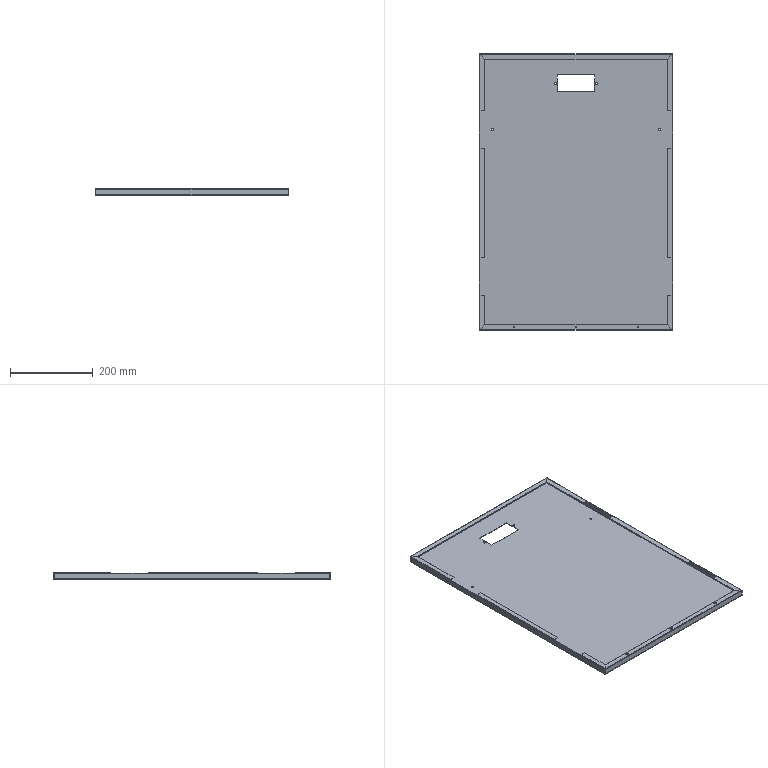Part | STEP file | 1 solid | 165 faces | box 467 x 667 x 16 mm | volume 433959 mm3 | plane 109 | cylinder 48 | spline 8 | commonest cylinder face diameters 0.02 x16 2.42 x12 5 x8 3.3 x6 8 x6